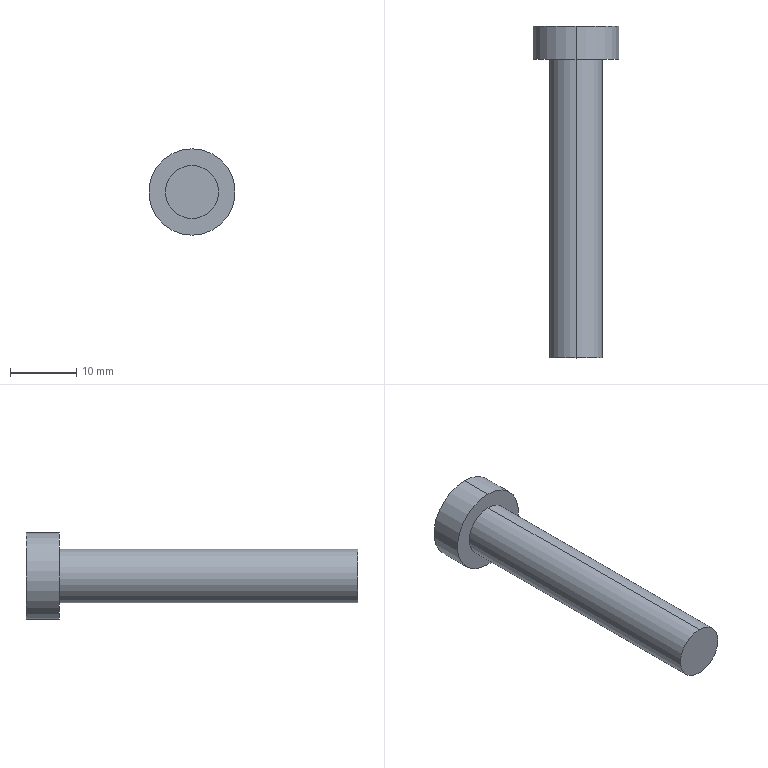Part | SolidWorks | features Revolution 1 | 1 solid | 7 faces | box 13 x 50 x 13 mm | volume 2926 mm3 | cylinder 4 | plane 3 | commonest cylinder face diameters 8 x2 13 x2
STEP:
#1=CARTESIAN_POINT('',(0.,45.,-4.));
#2=VERTEX_POINT('',#1);
#3=CARTESIAN_POINT('',(0.,45.,4.));
#4=VERTEX_POINT('',#3);
#5=CARTESIAN_POINT('',(0.,45.,0.));
#6=DIRECTION('',(0.,-1.,0.));
#7=DIRECTION('',(0.,0.,-1.));
#8=AXIS2_PLACEMENT_3D('',#5,#6,#7);
#9=CIRCLE('',#8,4.);
#10=EDGE_CURVE('',#2,#4,#9,.T.);
#11=ORIENTED_EDGE('',*,*,#10,.T.);
#12=CARTESIAN_POINT('',(0.,0.,4.));
#13=VERTEX_POINT('',#12);
#14=CARTESIAN_POINT('',(0.,0.,4.));
#15=DIRECTION('',(0.,-1.,0.));
#16=VECTOR('',#15,1000.);
#17=LINE('',#14,#16);
#18=EDGE_CURVE('',#4,#13,#17,.T.);
#19=ORIENTED_EDGE('',*,*,#18,.T.);
#20=CARTESIAN_POINT('',(0.,0.,-4.));
#21=VERTEX_POINT('',#20);
#22=CARTESIAN_POINT('',(0.,0.,0.));
#23=DIRECTION('',(0.,-1.,0.));
#24=DIRECTION('',(0.,0.,-1.));
#25=AXIS2_PLACEMENT_3D('',#22,#23,#24);
#26=CIRCLE('',#25,4.);
#27=EDGE_CURVE('',#21,#13,#26,.T.);
#28=ORIENTED_EDGE('',*,*,#27,.F.);
#29=CARTESIAN_POINT('',(0.,0.,-4.));
#30=DIRECTION('',(0.,-1.,0.));
#31=VECTOR('',#30,1000.);
#32=LINE('',#29,#31);
#33=EDGE_CURVE('',#2,#21,#32,.T.);
#34=ORIENTED_EDGE('',*,*,#33,.F.);
#35=EDGE_LOOP('',(#11,#19,#28,#34));
#36=FACE_OUTER_BOUND('',#35,.T.);
#37=CARTESIAN_POINT('',(0.,0.,0.));
#38=DIRECTION('',(0.,-1.,0.));
#39=DIRECTION('',(0.,0.,-1.));
#40=AXIS2_PLACEMENT_3D('',#37,#38,#39);
#41=CYLINDRICAL_SURFACE('',#40,4.);
#42=ADVANCED_FACE('',(#36),#41,.T.);
#43=CARTESIAN_POINT('',(0.,50.,-6.5));
#44=VERTEX_POINT('',#43);
#45=CARTESIAN_POINT('',(0.,50.,6.5));
#46=VERTEX_POINT('',#45);
#47=CARTESIAN_POINT('',(0.,50.,0.));
#48=DIRECTION('',(0.,-1.,0.));
#49=DIRECTION('',(0.,0.,-1.));
#50=AXIS2_PLACEMENT_3D('',#47,#48,#49);
#51=CIRCLE('',#50,6.5);
#52=EDGE_CURVE('',#44,#46,#51,.T.);
#53=ORIENTED_EDGE('',*,*,#52,.T.);
#54=CARTESIAN_POINT('',(0.,45.,6.5));
#55=VERTEX_POINT('',#54);
#56=CARTESIAN_POINT('',(0.,0.,6.5));
#57=DIRECTION('',(0.,-1.,0.));
#58=VECTOR('',#57,1000.);
#59=LINE('',#56,#58);
#60=EDGE_CURVE('',#46,#55,#59,.T.);
#61=ORIENTED_EDGE('',*,*,#60,.T.);
#62=CARTESIAN_POINT('',(0.,45.,-6.5));
#63=VERTEX_POINT('',#62);
#64=CARTESIAN_POINT('',(0.,45.,0.));
#65=DIRECTION('',(0.,-1.,0.));
#66=DIRECTION('',(0.,0.,-1.));
#67=AXIS2_PLACEMENT_3D('',#64,#65,#66);
#68=CIRCLE('',#67,6.5);
#69=EDGE_CURVE('',#63,#55,#68,.T.);
#70=ORIENTED_EDGE('',*,*,#69,.F.);
#71=CARTESIAN_POINT('',(0.,0.,-6.5));
#72=DIRECTION('',(0.,-1.,0.));
#73=VECTOR('',#72,1000.);
#74=LINE('',#71,#73);
#75=EDGE_CURVE('',#44,#63,#74,.T.);
#76=ORIENTED_EDGE('',*,*,#75,.F.);
#77=EDGE_LOOP('',(#53,#61,#70,#76));
#78=FACE_OUTER_BOUND('',#77,.T.);
#79=CARTESIAN_POINT('',(0.,0.,0.));
#80=DIRECTION('',(0.,-1.,0.));
#81=DIRECTION('',(0.,0.,-1.));
#82=AXIS2_PLACEMENT_3D('',#79,#80,#81);
#83=CYLINDRICAL_SURFACE('',#82,6.5);
#84=ADVANCED_FACE('',(#78),#83,.T.);
#85=ORIENTED_EDGE('',*,*,#27,.T.);
#86=CARTESIAN_POINT('',(0.,0.,0.));
#87=DIRECTION('',(0.,-1.,0.));
#88=DIRECTION('',(0.,0.,-1.));
#89=AXIS2_PLACEMENT_3D('',#86,#87,#88);
#90=CIRCLE('',#89,4.);
#91=EDGE_CURVE('',#13,#21,#90,.T.);
#92=ORIENTED_EDGE('',*,*,#91,.T.);
#93=EDGE_LOOP('',(#85,#92));
#94=FACE_OUTER_BOUND('',#93,.T.);
#95=CARTESIAN_POINT('',(4.,0.,0.));
#96=DIRECTION('',(0.,-1.,0.));
#97=DIRECTION('',(0.,0.,-1.));
#98=AXIS2_PLACEMENT_3D('',#95,#96,#97);
#99=PLANE('',#98);
#100=ADVANCED_FACE('',(#94),#99,.T.);
#101=ORIENTED_EDGE('',*,*,#52,.F.);
#102=CARTESIAN_POINT('',(0.,50.,0.));
#103=DIRECTION('',(0.,-1.,0.));
#104=DIRECTION('',(0.,0.,-1.));
#105=AXIS2_PLACEMENT_3D('',#102,#103,#104);
#106=CIRCLE('',#105,6.5);
#107=EDGE_CURVE('',#46,#44,#106,.T.);
#108=ORIENTED_EDGE('',*,*,#107,.F.);
#109=EDGE_LOOP('',(#101,#108));
#110=FACE_OUTER_BOUND('',#109,.T.);
#111=CARTESIAN_POINT('',(0.,50.,0.));
#112=DIRECTION('',(0.,1.,0.));
#113=DIRECTION('',(0.,0.,1.));
#114=AXIS2_PLACEMENT_3D('',#111,#112,#113);
#115=PLANE('',#114);
#116=ADVANCED_FACE('',(#110),#115,.T.);
#117=ORIENTED_EDGE('',*,*,#60,.F.);
#118=ORIENTED_EDGE('',*,*,#107,.T.);
#119=ORIENTED_EDGE('',*,*,#75,.T.);
#120=CARTESIAN_POINT('',(0.,45.,0.));
#121=DIRECTION('',(0.,-1.,0.));
#122=DIRECTION('',(0.,0.,-1.));
#123=AXIS2_PLACEMENT_3D('',#120,#121,#122);
#124=CIRCLE('',#123,6.5);
#125=EDGE_CURVE('',#55,#63,#124,.T.);
#126=ORIENTED_EDGE('',*,*,#125,.F.);
#127=EDGE_LOOP('',(#117,#118,#119,#126));
#128=FACE_OUTER_BOUND('',#127,.T.);
#129=CARTESIAN_POINT('',(0.,0.,0.));
#130=DIRECTION('',(0.,-1.,0.));
#131=DIRECTION('',(0.,0.,-1.));
#132=AXIS2_PLACEMENT_3D('',#129,#130,#131);
#133=CYLINDRICAL_SURFACE('',#132,6.5);
#134=ADVANCED_FACE('',(#128),#133,.T.);
#135=ORIENTED_EDGE('',*,*,#69,.T.);
#136=ORIENTED_EDGE('',*,*,#125,.T.);
#137=EDGE_LOOP('',(#135,#136));
#138=FACE_OUTER_BOUND('',#137,.T.);
#139=ORIENTED_EDGE('',*,*,#10,.F.);
#140=CARTESIAN_POINT('',(0.,45.,0.));
#141=DIRECTION('',(0.,-1.,0.));
#142=DIRECTION('',(0.,0.,-1.));
#143=AXIS2_PLACEMENT_3D('',#140,#141,#142);
#144=CIRCLE('',#143,4.);
#145=EDGE_CURVE('',#4,#2,#144,.T.);
#146=ORIENTED_EDGE('',*,*,#145,.F.);
#147=EDGE_LOOP('',(#139,#146));
#148=FACE_BOUND('',#147,.T.);
#149=CARTESIAN_POINT('',(6.5,45.,0.));
#150=DIRECTION('',(0.,-1.,0.));
#151=DIRECTION('',(0.,0.,-1.));
#152=AXIS2_PLACEMENT_3D('',#149,#150,#151);
#153=PLANE('',#152);
#154=ADVANCED_FACE('',(#138,#148),#153,.T.);
#155=ORIENTED_EDGE('',*,*,#18,.F.);
#156=ORIENTED_EDGE('',*,*,#145,.T.);
#157=ORIENTED_EDGE('',*,*,#33,.T.);
#158=ORIENTED_EDGE('',*,*,#91,.F.);
#159=EDGE_LOOP('',(#155,#156,#157,#158));
#160=FACE_OUTER_BOUND('',#159,.T.);
#161=CARTESIAN_POINT('',(0.,0.,0.));
#162=DIRECTION('',(0.,-1.,0.));
#163=DIRECTION('',(0.,0.,-1.));
#164=AXIS2_PLACEMENT_3D('',#161,#162,#163);
#165=CYLINDRICAL_SURFACE('',#164,4.);
#166=ADVANCED_FACE('',(#160),#165,.T.);
#167=CLOSED_SHELL('',(#42,#84,#100,#116,#134,#154,#166));
#168=MANIFOLD_SOLID_BREP('',#167);
#169=CARTESIAN_POINT('',(0.,0.,0.));
#170=DIRECTION('',(0.,0.,1.));
#171=DIRECTION('',(1.,0.,0.));
#172=AXIS2_PLACEMENT_3D('',#169,#170,#171);
#173=(LENGTH_UNIT()NAMED_UNIT(*)SI_UNIT(.MILLI.,.METRE.));
#174=UNCERTAINTY_MEASURE_WITH_UNIT(LENGTH_MEASURE(0.00001),#173,'','');
#175=(NAMED_UNIT(*)PLANE_ANGLE_UNIT()SI_UNIT($,.RADIAN.));
#176=(NAMED_UNIT(*)SI_UNIT($,.STERADIAN.)SOLID_ANGLE_UNIT());
#177=(GEOMETRIC_REPRESENTATION_CONTEXT(3)GLOBAL_UNCERTAINTY_ASSIGNED_CONTEXT((#174))GLOBAL_UNIT_ASSIGNED_CONTEXT((#173,#175,#176))REPRESENTATION_CONTEXT('',''));
#178=ADVANCED_BREP_SHAPE_REPRESENTATION('',(#168,#172),#177);